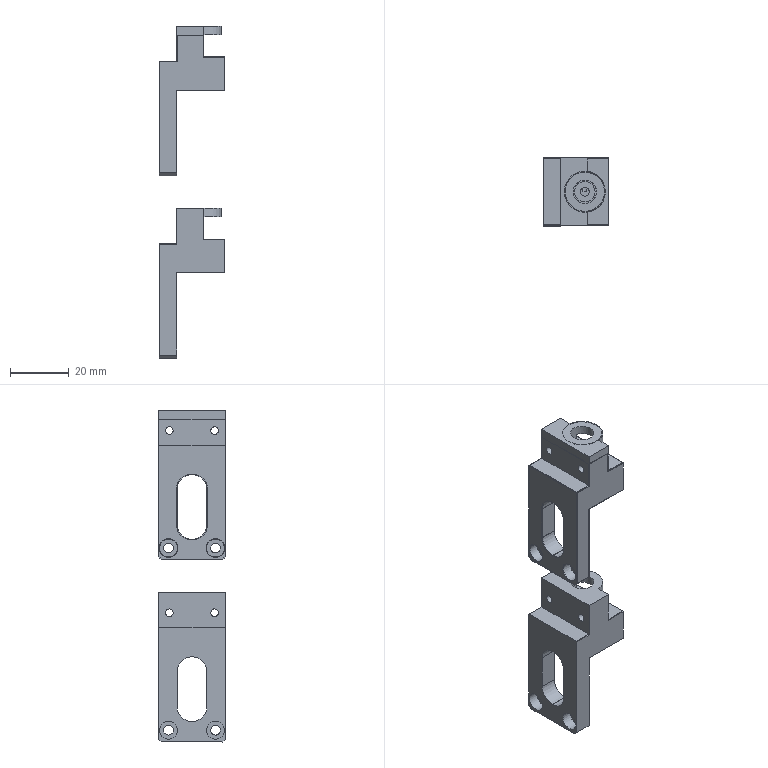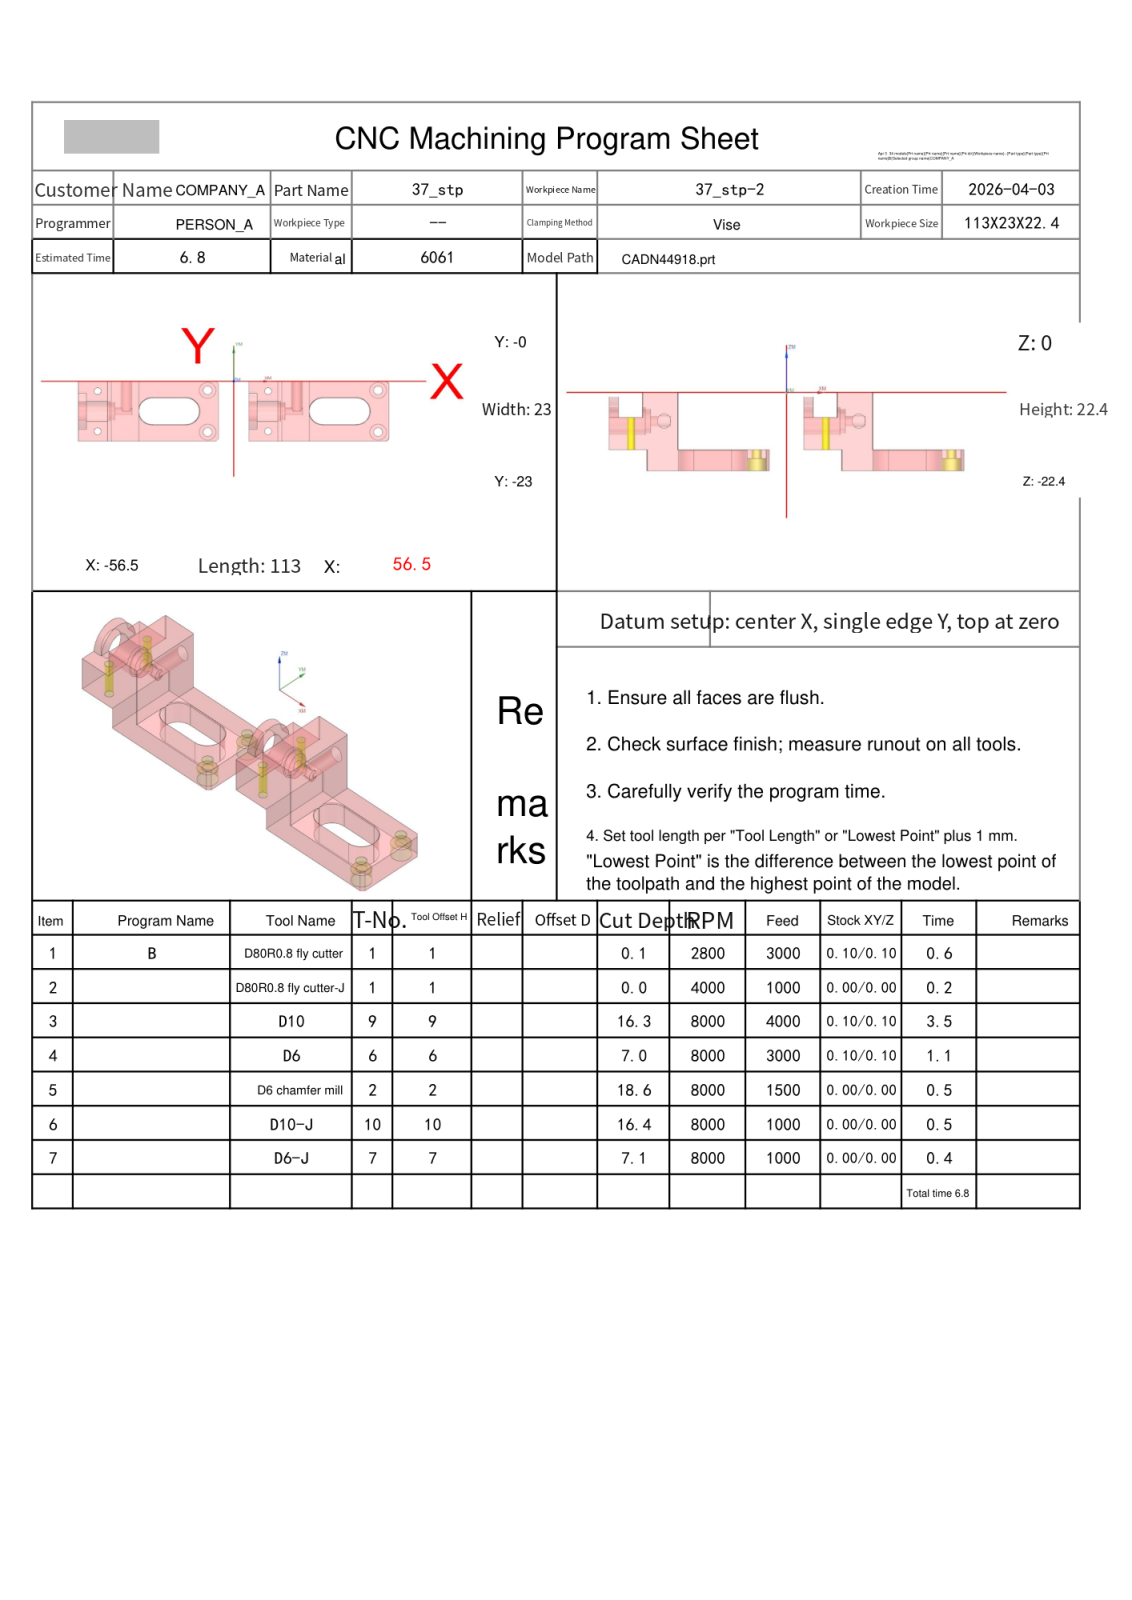NC program | NX | posted by the shop | part box 22.4 x 23 x 113 mm
Lines 1 to 3243 of 3535, first 2166 of 3241 lines:
%
O0001
(Machine time: 8.11 MIN)
(===Total Tool:6===)
(T1=D80R0.8 fly cutter D=80.  R=0.8  D-  H01 Z=-0.   )
(T9=D10     D=10.  R=0.   D-  H09 Z=-16.3 )
(T6=D6      D=6.   R=0.   D-  H06 Z=-7.05 )
(T2=D6 chamfer mill   D=6.   R=0.   D-  H02 Z=-18.6 )
(T10=D10-J  D=10.  R=0.   D10 H10 Z=-16.4 )
(T7=D6-J    D=6.   R=0.   D7  H07 Z=-7.15 )
G80 G90 G17 G49 G40
G91 G28 Z0
M01
N1 T01 M06
(D80R0.8 fly cutter  D=80. R=0.8 H=01 ce=0.10 di=0.10)
G00 G90 G54 X-108.597 Y-11.5 M03 S2800
G43 H01 Z20.
M08
Z4.517
G01 Z2.517 F3000.
X-96.597
X96.597
X108.597
Z4.517
G00 X-108.597
Z4.033
G01 Z2.033
X-96.597
X96.597
X108.597
Z4.033
G00 X-108.597
Z3.55
G01 Z1.55
X-96.597
X96.597
X108.597
Z3.55
G00 X-108.597
Z3.067
G01 Z1.067
X-96.597
X96.597
X108.597
Z3.067
G00 Z20.
X-108.597
Z2.583
G01 Z.583
X-96.597
X96.597
X108.597
Z2.583
G00 Z20.
X-108.597
Z2.1
G01 Z.1
X-96.597
X96.597
X108.597
Z2.1
G00 Z20.
G91 G28 Z0.0
M05
M09
G91 G28 Z0.0
M01
N2 T01 M06
(D80R0.8 fly cutter-J  D=80. R=0.8 H=01 ce=0.00 di=0.00)
G00 G90 G54 X-108.499 Y-11.5 M03 S4000
G43 H01 Z20.
M08
Z2.
G01 Z0.0 F1000.
X-96.499
X96.499
X108.499
Z2.
G00 Z20.
G91 G28 Z0.0
M05
M09
G91 G28 Z0.0
M01
N3 T09 M06
(D10  D=10. R=0. H=09 ce=0.10 di=0.10)
G00 G90 G54 X64.5 Y-11.5 M03 S8000
G43 H09 Z12.4
M08
Z.918
G01 Z-.582 F4000.
X61.4
Y-24.03
X57.53 Y-27.9
X29.612
X32.6 Y-24.912
Y-11.9
X44.5
G03 X44.8 Y-11.6 I0.0 J.3
G01 Y-11.4
G03 X44.5 Y-11.1 I-.3 J0.0
G01 X32.6
Y1.912
X29.612 Y4.9
X57.53
X61.4 Y1.03
Y-8.465
G02 X60.955 Y-9.297 I-1. J0.0
G01 X54.345 Y-13.703
G03 X53.9 Y-14.535 I.555 J-.832
G01 Y-19.401
G02 X52.901 Y-20.4 I-1. J.001
G01 X40.599
G02 X40.1 Y-19.9 I.001 J.5
X40.599 Y-19.4 I.5 J0.0
G01 X44.5
G03 X52.3 Y-11.6 I0.0 J7.8
X52.303 Y-11.4 I-7.797 J.2
X44.503 Y-3.6 I-7.8 J0.0
G01 X44.5
X40.599
G02 X40.1 Y-3.1 I.001 J.5
X40.599 Y-2.6 I.5 J0.0
G01 X52.901
G02 X53.9 Y-3.599 I-.001 J-1.
G01 Y-11.5
Y-12.
X64.5
Z.918
G00 Y-11.5
Z.336
G01 Z-1.164
X61.4
Y-24.03
X57.53 Y-27.9
X29.612
X32.6 Y-24.912
Y-11.9
X44.5
G03 X44.8 Y-11.6 I0.0 J.3
G01 Y-11.4
G03 X44.5 Y-11.1 I-.3 J0.0
G01 X32.6
Y1.912
X29.612 Y4.9
X57.53
X61.4 Y1.03
Y-8.465
G02 X60.955 Y-9.297 I-1. J0.0
G01 X54.345 Y-13.703
G03 X53.9 Y-14.535 I.555 J-.832
G01 Y-19.401
G02 X52.901 Y-20.4 I-1. J.001
G01 X40.599
G02 X40.1 Y-19.9 I.001 J.5
X40.599 Y-19.4 I.5 J0.0
G01 X44.5
G03 X52.3 Y-11.6 I0.0 J7.8
X52.303 Y-11.4 I-7.797 J.2
X44.503 Y-3.6 I-7.8 J0.0
G01 X44.5
X40.599
G02 X40.1 Y-3.1 I.001 J.5
X40.599 Y-2.6 I.5 J0.0
G01 X52.901
G02 X53.9 Y-3.599 I-.001 J-1.
G01 Y-11.5
Y-12.
X64.5
Z.336
G00 Y-11.5
Z-.246
G01 Z-1.746
X61.4
Y-24.03
X57.53 Y-27.9
X29.612
X32.6 Y-24.912
Y-11.9
X44.5
G03 X44.8 Y-11.6 I0.0 J.3
G01 Y-11.4
G03 X44.5 Y-11.1 I-.3 J0.0
G01 X32.6
Y1.912
X29.612 Y4.9
X57.53
X61.4 Y1.03
Y-8.465
G02 X60.955 Y-9.297 I-1. J0.0
G01 X54.345 Y-13.703
G03 X53.9 Y-14.535 I.555 J-.832
G01 Y-19.401
G02 X52.901 Y-20.4 I-1. J.001
G01 X40.599
G02 X40.1 Y-19.9 I.001 J.5
X40.599 Y-19.4 I.5 J0.0
G01 X44.5
G03 X52.3 Y-11.6 I0.0 J7.8
X52.303 Y-11.4 I-7.797 J.2
X44.503 Y-3.6 I-7.8 J0.0
G01 X44.5
X40.599
G02 X40.1 Y-3.1 I.001 J.5
X40.599 Y-2.6 I.5 J0.0
G01 X52.901
G02 X53.9 Y-3.599 I-.001 J-1.
G01 Y-11.5
Y-12.
X64.5
Z-.246
G00 Y-11.5
Z-.829
G01 Z-2.329
X61.4
Y-24.03
X57.53 Y-27.9
X29.612
X32.6 Y-24.912
Y-11.9
X44.5
G03 X44.8 Y-11.6 I0.0 J.3
G01 Y-11.4
G03 X44.5 Y-11.1 I-.3 J0.0
G01 X32.6
Y1.912
X29.612 Y4.9
X57.53
X61.4 Y1.03
Y-8.465
G02 X60.955 Y-9.297 I-1. J0.0
G01 X54.345 Y-13.703
G03 X53.9 Y-14.535 I.555 J-.832
G01 Y-19.401
G02 X52.901 Y-20.4 I-1. J.001
G01 X40.599
G02 X40.1 Y-19.9 I.001 J.5
X40.599 Y-19.4 I.5 J0.0
G01 X44.5
G03 X52.3 Y-11.6 I0.0 J7.8
X52.303 Y-11.4 I-7.797 J.2
X44.503 Y-3.6 I-7.8 J0.0
G01 X44.5
X40.599
G02 X40.1 Y-3.1 I.001 J.5
X40.599 Y-2.6 I.5 J0.0
G01 X52.901
G02 X53.9 Y-3.599 I-.001 J-1.
G01 Y-11.5
Y-12.
X64.5
Z-.829
G00 Y-11.5
Z-1.411
G01 Z-2.911
X61.4
Y-24.03
X57.53 Y-27.9
X29.612
X32.6 Y-24.912
Y-11.9
X44.5
G03 X44.8 Y-11.6 I0.0 J.3
G01 Y-11.4
G03 X44.5 Y-11.1 I-.3 J0.0
G01 X32.6
Y1.912
X29.612 Y4.9
X57.53
X61.4 Y1.03
Y-8.465
G02 X60.955 Y-9.297 I-1. J0.0
G01 X54.345 Y-13.703
G03 X53.9 Y-14.535 I.555 J-.832
G01 Y-19.401
G02 X52.901 Y-20.4 I-1. J.001
G01 X40.599
G02 X40.1 Y-19.9 I.001 J.5
X40.599 Y-19.4 I.5 J0.0
G01 X44.5
G03 X52.3 Y-11.6 I0.0 J7.8
X52.303 Y-11.4 I-7.797 J.2
X44.503 Y-3.6 I-7.8 J0.0
G01 X44.5
X40.599
G02 X40.1 Y-3.1 I.001 J.5
X40.599 Y-2.6 I.5 J0.0
G01 X52.901
G02 X53.9 Y-3.599 I-.001 J-1.
G01 Y-11.5
Y-12.
X64.5
Z-1.411
G00 Y-11.5
Z-1.993
G01 Z-3.493
X61.4
Y-24.03
X57.53 Y-27.9
X29.612
X32.6 Y-24.912
Y-11.9
X44.5
G03 X44.8 Y-11.6 I0.0 J.3
G01 Y-11.4
G03 X44.5 Y-11.1 I-.3 J0.0
G01 X32.6
Y1.912
X29.612 Y4.9
X57.53
X61.4 Y1.03
Y-8.465
G02 X60.955 Y-9.297 I-1. J0.0
G01 X54.345 Y-13.703
G03 X53.9 Y-14.535 I.555 J-.832
G01 Y-19.401
G02 X52.901 Y-20.4 I-1. J.001
G01 X40.599
G02 X40.1 Y-19.9 I.001 J.5
X40.599 Y-19.4 I.5 J0.0
G01 X44.5
G03 X52.3 Y-11.6 I0.0 J7.8
X52.303 Y-11.4 I-7.797 J.2
X44.503 Y-3.6 I-7.8 J0.0
G01 X44.5
X40.599
G02 X40.1 Y-3.1 I.001 J.5
X40.599 Y-2.6 I.5 J0.0
G01 X52.901
G02 X53.9 Y-3.599 I-.001 J-1.
G01 Y-11.5
Y-12.
X64.5
Z-1.993
G00 Y-11.5
Z-2.575
G01 Z-4.075
X61.4
Y-24.03
X57.53 Y-27.9
X29.612
X32.6 Y-24.912
Y-11.9
X44.5
G03 X44.8 Y-11.6 I0.0 J.3
G01 Y-11.4
G03 X44.5 Y-11.1 I-.3 J0.0
G01 X32.6
Y1.912
X29.612 Y4.9
X57.53
X61.4 Y1.03
Y-8.465
G02 X60.955 Y-9.297 I-1. J0.0
G01 X54.345 Y-13.703
G03 X53.9 Y-14.535 I.555 J-.832
G01 Y-19.401
G02 X52.901 Y-20.4 I-1. J.001
G01 X40.599
G02 X40.1 Y-19.9 I.001 J.5
X40.599 Y-19.4 I.5 J0.0
G01 X44.5
G03 X52.3 Y-11.6 I0.0 J7.8
X52.303 Y-11.4 I-7.797 J.2
X44.503 Y-3.6 I-7.8 J0.0
G01 X44.5
X40.599
G02 X40.1 Y-3.1 I.001 J.5
X40.599 Y-2.6 I.5 J0.0
G01 X52.901
G02 X53.9 Y-3.599 I-.001 J-1.
G01 Y-11.5
Y-12.
X64.5
Z-2.575
G00 Y-11.5
Z-3.157
G01 Z-4.657
X61.4
Y-24.03
X57.53 Y-27.9
X29.612
X32.6 Y-24.912
Y-11.9
X44.5
G03 X44.8 Y-11.6 I0.0 J.3
G01 Y-11.4
G03 X44.5 Y-11.1 I-.3 J0.0
G01 X32.6
Y1.912
X29.612 Y4.9
X57.53
X61.4 Y1.03
Y-8.465
G02 X60.955 Y-9.297 I-1. J0.0
G01 X54.345 Y-13.703
G03 X53.9 Y-14.535 I.555 J-.832
G01 Y-19.401
G02 X52.901 Y-20.4 I-1. J.001
G01 X40.599
G02 X40.1 Y-19.9 I.001 J.5
X40.599 Y-19.4 I.5 J0.0
G01 X44.5
G03 X52.3 Y-11.6 I0.0 J7.8
X52.303 Y-11.4 I-7.797 J.2
X44.503 Y-3.6 I-7.8 J0.0
G01 X44.5
X40.599
G02 X40.1 Y-3.1 I.001 J.5
X40.599 Y-2.6 I.5 J0.0
G01 X52.901
G02 X53.9 Y-3.599 I-.001 J-1.
G01 Y-11.5
Y-12.
X64.5
Z-3.157
G00 Y-11.5
Z-3.739
G01 Z-5.239
X61.4
Y-24.03
X57.53 Y-27.9
X29.612
X32.6 Y-24.912
Y-11.9
X44.5
G03 X44.8 Y-11.6 I0.0 J.3
G01 Y-11.4
G03 X44.5 Y-11.1 I-.3 J0.0
G01 X32.6
Y1.912
X29.612 Y4.9
X57.53
X61.4 Y1.03
Y-8.465
G02 X60.955 Y-9.297 I-1. J0.0
G01 X54.345 Y-13.703
G03 X53.9 Y-14.535 I.555 J-.832
G01 Y-19.401
G02 X52.901 Y-20.4 I-1. J.001
G01 X40.599
G02 X40.1 Y-19.9 I.001 J.5
X40.599 Y-19.4 I.5 J0.0
G01 X44.5
G03 X52.3 Y-11.6 I0.0 J7.8
X52.303 Y-11.4 I-7.797 J.2
X44.503 Y-3.6 I-7.8 J0.0
G01 X44.5
X40.599
G02 X40.1 Y-3.1 I.001 J.5
X40.599 Y-2.6 I.5 J0.0
G01 X52.901
G02 X53.9 Y-3.599 I-.001 J-1.
G01 Y-11.5
Y-12.
X64.5
Z-3.739
G00 Y-11.5
Z-4.321
G01 Z-5.821
X61.4
Y-24.03
X57.53 Y-27.9
X29.612
X32.6 Y-24.912
Y-11.9
X44.5
G03 X44.8 Y-11.6 I0.0 J.3
G01 Y-11.4
G03 X44.5 Y-11.1 I-.3 J0.0
G01 X32.6
Y1.912
X29.612 Y4.9
X57.53
X61.4 Y1.03
Y-8.465
G02 X60.955 Y-9.297 I-1. J0.0
G01 X54.345 Y-13.703
G03 X53.9 Y-14.535 I.555 J-.832
G01 Y-19.401
G02 X52.901 Y-20.4 I-1. J.001
G01 X40.599
G02 X40.1 Y-19.9 I.001 J.5
X40.599 Y-19.4 I.5 J0.0
G01 X44.5
G03 X52.3 Y-11.6 I0.0 J7.8
X52.303 Y-11.4 I-7.797 J.2
X44.503 Y-3.6 I-7.8 J0.0
G01 X44.5
X40.599
G02 X40.1 Y-3.1 I.001 J.5
X40.599 Y-2.6 I.5 J0.0
G01 X52.901
G02 X53.9 Y-3.599 I-.001 J-1.
G01 Y-11.5
Y-12.
X64.5
Z-4.321
G00 Y-11.5
Z-4.904
G01 Z-6.404
X61.4
Y-24.03
X57.53 Y-27.9
X29.612
X32.6 Y-24.912
Y-11.9
X44.5
G03 X44.8 Y-11.6 I0.0 J.3
G01 Y-11.4
G03 X44.5 Y-11.1 I-.3 J0.0
G01 X32.6
Y1.912
X29.612 Y4.9
X57.53
X61.4 Y1.03
Y-8.465
G02 X60.955 Y-9.297 I-1. J0.0
G01 X54.345 Y-13.703
G03 X53.9 Y-14.535 I.555 J-.832
G01 Y-19.401
G02 X52.901 Y-20.4 I-1. J.001
G01 X40.599
G02 X40.1 Y-19.9 I.001 J.5
X40.599 Y-19.4 I.5 J0.0
G01 X44.5
G03 X52.3 Y-11.6 I0.0 J7.8
X52.303 Y-11.4 I-7.797 J.2
X44.503 Y-3.6 I-7.8 J0.0
G01 X44.5
X40.599
G02 X40.1 Y-3.1 I.001 J.5
X40.599 Y-2.6 I.5 J0.0
G01 X52.901
G02 X53.9 Y-3.599 I-.001 J-1.
G01 Y-11.5
Y-12.
X64.5
Z-4.904
G00 Y-11.5
Z-5.486
G01 Z-6.986
X61.4
Y-24.03
X57.53 Y-27.9
X29.612
X32.6 Y-24.912
Y-11.9
X44.5
G03 X44.8 Y-11.6 I0.0 J.3
G01 Y-11.4
G03 X44.5 Y-11.1 I-.3 J0.0
G01 X32.6
Y1.912
X29.612 Y4.9
X57.53
X61.4 Y1.03
Y-8.465
G02 X60.955 Y-9.297 I-1. J0.0
G01 X54.345 Y-13.703
G03 X53.9 Y-14.535 I.555 J-.832
G01 Y-19.401
G02 X52.901 Y-20.4 I-1. J.001
G01 X40.599
G02 X40.1 Y-19.9 I.001 J.5
X40.599 Y-19.4 I.5 J0.0
G01 X44.5
G03 X52.3 Y-11.6 I0.0 J7.8
X52.303 Y-11.4 I-7.797 J.2
X44.503 Y-3.6 I-7.8 J0.0
G01 X44.5
X40.599
G02 X40.1 Y-3.1 I.001 J.5
X40.599 Y-2.6 I.5 J0.0
G01 X52.901
G02 X53.9 Y-3.599 I-.001 J-1.
G01 Y-11.5
Y-12.
X64.5
Z-5.486
G00 Y-11.5
Z-6.068
G01 Z-7.568
X61.4
Y-24.03
X57.53 Y-27.9
X29.612
X32.6 Y-24.912
Y-11.9
X44.5
G03 X44.8 Y-11.6 I0.0 J.3
G01 Y-11.4
G03 X44.5 Y-11.1 I-.3 J0.0
G01 X32.6
Y1.912
X29.612 Y4.9
X57.53
X61.4 Y1.03
Y-8.465
G02 X60.955 Y-9.297 I-1. J0.0
G01 X54.345 Y-13.703
G03 X53.9 Y-14.535 I.555 J-.832
G01 Y-19.401
G02 X52.901 Y-20.4 I-1. J.001
G01 X40.599
G02 X40.1 Y-19.9 I.001 J.5
X40.599 Y-19.4 I.5 J0.0
G01 X44.5
G03 X52.3 Y-11.6 I0.0 J7.8
X52.303 Y-11.4 I-7.797 J.2
X44.503 Y-3.6 I-7.8 J0.0
G01 X44.5
X40.599
G02 X40.1 Y-3.1 I.001 J.5
X40.599 Y-2.6 I.5 J0.0
G01 X52.901
G02 X53.9 Y-3.599 I-.001 J-1.
G01 Y-11.5
Y-12.
X64.5
Z-6.068
G00 Y-11.5
Z-6.65
G01 Z-8.15
X61.4
Y-24.03
X57.53 Y-27.9
X29.612
X32.6 Y-24.912
Y-11.9
X44.5
G03 X44.8 Y-11.6 I0.0 J.3
G01 Y-11.4
G03 X44.5 Y-11.1 I-.3 J0.0
G01 X32.6
Y1.912
X29.612 Y4.9
X57.53
X61.4 Y1.03
Y-8.465
G02 X60.955 Y-9.297 I-1. J0.0
G01 X54.345 Y-13.703
G03 X53.9 Y-14.535 I.555 J-.832
G01 Y-19.401
G02 X52.901 Y-20.4 I-1. J.001
G01 X40.599
G02 X40.1 Y-19.9 I.001 J.5
X40.599 Y-19.4 I.5 J0.0
G01 X44.5
G03 X52.3 Y-11.6 I0.0 J7.8
X52.303 Y-11.4 I-7.797 J.2
X44.503 Y-3.6 I-7.8 J0.0
G01 X44.5
X40.599
G02 X40.1 Y-3.1 I.001 J.5
X40.599 Y-2.6 I.5 J0.0
G01 X52.901
G02 X53.9 Y-3.599 I-.001 J-1.
G01 Y-11.5
Y-12.
X64.5
Z-6.65
G00 Y-11.5
Z-7.232
G01 Z-8.732
X61.4
Y-24.03
X57.53 Y-27.9
X29.612
X32.6 Y-24.912
Y-11.9
X44.5
G03 X44.8 Y-11.6 I0.0 J.3
G01 Y-11.4
G03 X44.5 Y-11.1 I-.3 J0.0
G01 X32.6
Y1.912
X29.612 Y4.9
X57.53
X61.4 Y1.03
Y-8.465
G02 X60.955 Y-9.297 I-1. J0.0
G01 X54.345 Y-13.703
G03 X53.9 Y-14.535 I.555 J-.832
G01 Y-19.401
G02 X52.901 Y-20.4 I-1. J.001
G01 X40.599
G02 X40.1 Y-19.9 I.001 J.5
X40.599 Y-19.4 I.5 J0.0
G01 X44.5
G03 X52.3 Y-11.6 I0.0 J7.8
X52.303 Y-11.4 I-7.797 J.2
X44.503 Y-3.6 I-7.8 J0.0
G01 X44.5
X40.599
G02 X40.1 Y-3.1 I.001 J.5
X40.599 Y-2.6 I.5 J0.0
G01 X52.901
G02 X53.9 Y-3.599 I-.001 J-1.
G01 Y-11.5
Y-12.
X64.5
Z-7.232
G00 Y-11.5
Z-7.814
G01 Z-9.314
X61.4
Y-24.03
X57.53 Y-27.9
X29.612
X32.6 Y-24.912
Y-11.9
X44.5
G03 X44.8 Y-11.6 I0.0 J.3
G01 Y-11.4
G03 X44.5 Y-11.1 I-.3 J0.0
G01 X32.6
Y1.912
X29.612 Y4.9
X57.53
X61.4 Y1.03
Y-8.465
G02 X60.955 Y-9.297 I-1. J0.0
G01 X54.345 Y-13.703
G03 X53.9 Y-14.535 I.555 J-.832
G01 Y-19.401
G02 X52.901 Y-20.4 I-1. J.001
G01 X40.599
G02 X40.1 Y-19.9 I.001 J.5
X40.599 Y-19.4 I.5 J0.0
G01 X44.5
G03 X52.3 Y-11.6 I0.0 J7.8
X52.303 Y-11.4 I-7.797 J.2
X44.503 Y-3.6 I-7.8 J0.0
G01 X44.5
X40.599
G02 X40.1 Y-3.1 I.001 J.5
X40.599 Y-2.6 I.5 J0.0
G01 X52.901
G02 X53.9 Y-3.599 I-.001 J-1.
G01 Y-11.5
Y-12.
X64.5
Z-7.814
G00 Y-11.5
Z-8.396
G01 Z-9.896
X61.4
Y-24.03
X57.53 Y-27.9
X29.612
X32.6 Y-24.912
Y-11.9
X44.5
G03 X44.8 Y-11.6 I0.0 J.3
G01 Y-11.4
G03 X44.5 Y-11.1 I-.3 J0.0
G01 X32.6
Y1.912
X29.612 Y4.9
X57.53
X61.4 Y1.03
Y-8.465
G02 X60.955 Y-9.297 I-1. J0.0
G01 X54.345 Y-13.703
G03 X53.9 Y-14.535 I.555 J-.832
G01 Y-19.401
G02 X52.901 Y-20.4 I-1. J.001
G01 X40.599
G02 X40.1 Y-19.9 I.001 J.5
X40.599 Y-19.4 I.5 J0.0
G01 X44.5
G03 X52.3 Y-11.6 I0.0 J7.8
X52.303 Y-11.4 I-7.797 J.2
X44.503 Y-3.6 I-7.8 J0.0
G01 X44.5
X40.599
G02 X40.1 Y-3.1 I.001 J.5
X40.599 Y-2.6 I.5 J0.0
G01 X52.901
G02 X53.9 Y-3.599 I-.001 J-1.
G01 Y-11.5
Y-12.
X64.5
Z-8.396
G00 Y-11.5
Z-8.979
G01 Z-10.479
X61.4
Y-24.03
X57.53 Y-27.9
X29.612
X32.6 Y-24.912
Y-11.9
X44.5
G03 X44.8 Y-11.6 I0.0 J.3
G01 Y-11.4
G03 X44.5 Y-11.1 I-.3 J0.0
G01 X32.6
Y1.912
X29.612 Y4.9
X57.53
X61.4 Y1.03
Y-8.465
G02 X60.955 Y-9.297 I-1. J0.0
G01 X54.345 Y-13.703
G03 X53.9 Y-14.535 I.555 J-.832
G01 Y-19.401
G02 X52.901 Y-20.4 I-1. J.001
G01 X40.599
G02 X40.1 Y-19.9 I.001 J.5
X40.599 Y-19.4 I.5 J0.0
G01 X44.5
G03 X52.3 Y-11.6 I0.0 J7.8
X52.303 Y-11.4 I-7.797 J.2
X44.503 Y-3.6 I-7.8 J0.0
G01 X44.5
X40.599
G02 X40.1 Y-3.1 I.001 J.5
X40.599 Y-2.6 I.5 J0.0
G01 X52.901
G02 X53.9 Y-3.599 I-.001 J-1.
G01 Y-11.5
Y-12.
X64.5
Z-8.979
G00 Y-11.5
Z-9.561
G01 Z-11.061
X61.4
Y-24.03
X57.53 Y-27.9
X29.612
X32.6 Y-24.912
Y-11.9
X44.5
G03 X44.8 Y-11.6 I0.0 J.3
G01 Y-11.4
G03 X44.5 Y-11.1 I-.3 J0.0
G01 X32.6
Y1.912
X29.612 Y4.9
X57.53
X61.4 Y1.03
Y-8.465
G02 X60.955 Y-9.297 I-1. J0.0
G01 X54.345 Y-13.703
G03 X53.9 Y-14.535 I.555 J-.832
G01 Y-19.401
G02 X52.901 Y-20.4 I-1. J.001
G01 X40.599
G02 X40.1 Y-19.9 I.001 J.5
X40.599 Y-19.4 I.5 J0.0
G01 X44.5
G03 X52.3 Y-11.6 I0.0 J7.8
X52.303 Y-11.4 I-7.797 J.2
X44.503 Y-3.6 I-7.8 J0.0
G01 X44.5
X40.599
G02 X40.1 Y-3.1 I.001 J.5
X40.599 Y-2.6 I.5 J0.0
G01 X52.901
G02 X53.9 Y-3.599 I-.001 J-1.
G01 Y-11.5
Y-12.
X64.5
Z-9.561
G00 Y-11.5
Z-10.143
G01 Z-11.643
X61.4
Y-24.03
X57.53 Y-27.9
X29.612
X32.6 Y-24.912
Y-11.9
X44.5
G03 X44.8 Y-11.6 I0.0 J.3
G01 Y-11.4
G03 X44.5 Y-11.1 I-.3 J0.0
G01 X32.6
Y1.912
X29.612 Y4.9
X57.53
X61.4 Y1.03
Y-8.465
G02 X60.955 Y-9.297 I-1. J0.0
G01 X54.345 Y-13.703
G03 X53.9 Y-14.535 I.555 J-.832
G01 Y-19.401
G02 X52.901 Y-20.4 I-1. J.001
G01 X40.599
G02 X40.1 Y-19.9 I.001 J.5
X40.599 Y-19.4 I.5 J0.0
G01 X44.5
G03 X52.3 Y-11.6 I0.0 J7.8
X52.303 Y-11.4 I-7.797 J.2
X44.503 Y-3.6 I-7.8 J0.0
G01 X44.5
X40.599
G02 X40.1 Y-3.1 I.001 J.5
X40.599 Y-2.6 I.5 J0.0
G01 X52.901
G02 X53.9 Y-3.599 I-.001 J-1.
G01 Y-11.5
Y-12.
X64.5
Z-10.143
G00 Y-11.5
Z-10.725
G01 Z-12.225
X61.4
Y-24.03
X57.53 Y-27.9
X29.612
X32.6 Y-24.912
Y-11.9
X44.5
G03 X44.8 Y-11.6 I0.0 J.3
G01 Y-11.4
G03 X44.5 Y-11.1 I-.3 J0.0
G01 X32.6
Y1.912
X29.612 Y4.9
X57.53
X61.4 Y1.03
Y-8.465
G02 X60.955 Y-9.297 I-1. J0.0
G01 X54.345 Y-13.703
G03 X53.9 Y-14.535 I.555 J-.832
G01 Y-19.401
G02 X52.901 Y-20.4 I-1. J.001
G01 X40.599
G02 X40.1 Y-19.9 I.001 J.5
X40.599 Y-19.4 I.5 J0.0
G01 X44.5
G03 X52.3 Y-11.6 I0.0 J7.8
X52.303 Y-11.4 I-7.797 J.2
X44.503 Y-3.6 I-7.8 J0.0
G01 X44.5
X40.599
G02 X40.1 Y-3.1 I.001 J.5
X40.599 Y-2.6 I.5 J0.0
G01 X52.901
G02 X53.9 Y-3.599 I-.001 J-1.
G01 Y-11.5
Y-12.
X64.5
Z-10.725
G00 Y-11.5
Z-11.307
G01 Z-12.807
X61.4
Y-24.03
X57.53 Y-27.9
X29.612
X32.6 Y-24.912
Y-11.9
X44.5
G03 X44.8 Y-11.6 I0.0 J.3
G01 Y-11.4
G03 X44.5 Y-11.1 I-.3 J0.0
G01 X32.6
Y1.912
X29.612 Y4.9
X57.53
X61.4 Y1.03
Y-8.465
G02 X60.955 Y-9.297 I-1. J0.0
G01 X54.345 Y-13.703
G03 X53.9 Y-14.535 I.555 J-.832
G01 Y-19.401
G02 X52.901 Y-20.4 I-1. J.001
G01 X40.599
G02 X40.1 Y-19.9 I.001 J.5
X40.599 Y-19.4 I.5 J0.0
G01 X44.5
G03 X52.3 Y-11.6 I0.0 J7.8
X52.303 Y-11.4 I-7.797 J.2
X44.503 Y-3.6 I-7.8 J0.0
G01 X44.5
X40.599
G02 X40.1 Y-3.1 I.001 J.5
X40.599 Y-2.6 I.5 J0.0
G01 X52.901
G02 X53.9 Y-3.599 I-.001 J-1.
G01 Y-11.5
Y-12.
X64.5
Z-11.307
G00 Y-11.5
Z-11.889
G01 Z-13.389
X61.4
Y-24.03
X57.53 Y-27.9
X29.612
X32.6 Y-24.912
Y-11.9
X44.5
G03 X44.8 Y-11.6 I0.0 J.3
G01 Y-11.4
G03 X44.5 Y-11.1 I-.3 J0.0
G01 X32.6
Y1.912
X29.612 Y4.9
X57.53
X61.4 Y1.03
Y-8.465
G02 X60.955 Y-9.297 I-1. J0.0
G01 X54.345 Y-13.703
G03 X53.9 Y-14.535 I.555 J-.832
G01 Y-19.401
G02 X52.901 Y-20.4 I-1. J.001
G01 X40.599
G02 X40.1 Y-19.9 I.001 J.5
X40.599 Y-19.4 I.5 J0.0
G01 X44.5
G03 X52.3 Y-11.6 I0.0 J7.8
X52.303 Y-11.4 I-7.797 J.2
X44.503 Y-3.6 I-7.8 J0.0
G01 X44.5
X40.599
G02 X40.1 Y-3.1 I.001 J.5
X40.599 Y-2.6 I.5 J0.0
G01 X52.901
G02 X53.9 Y-3.599 I-.001 J-1.
G01 Y-11.5
Y-12.
X64.5
Z-11.889
G00 Y-11.5
Z-12.471
G01 Z-13.971
X61.4
Y-24.03
X57.53 Y-27.9
X29.612
X32.6 Y-24.912
Y-11.9
X44.5
G03 X44.8 Y-11.6 I0.0 J.3
G01 Y-11.4
G03 X44.5 Y-11.1 I-.3 J0.0
G01 X32.6
Y1.912
X29.612 Y4.9
X57.53
X61.4 Y1.03
Y-8.465
G02 X60.955 Y-9.297 I-1. J0.0
G01 X54.345 Y-13.703
G03 X53.9 Y-14.535 I.555 J-.832
G01 Y-19.401
G02 X52.901 Y-20.4 I-1. J.001
G01 X40.599
G02 X40.1 Y-19.9 I.001 J.5
X40.599 Y-19.4 I.5 J0.0
G01 X44.5
G03 X52.3 Y-11.6 I0.0 J7.8
X52.303 Y-11.4 I-7.797 J.2
X44.503 Y-3.6 I-7.8 J0.0
G01 X44.5
X40.599
G02 X40.1 Y-3.1 I.001 J.5
X40.599 Y-2.6 I.5 J0.0
G01 X52.901
G02 X53.9 Y-3.599 I-.001 J-1.
G01 Y-11.5
Y-12.
X64.5
Z-12.471
G00 Y-11.5
Z-13.054
G01 Z-14.554
X61.4
Y-24.03
X57.53 Y-27.9
X29.612
X32.6 Y-24.912
Y-11.9
X44.5
G03 X44.8 Y-11.6 I0.0 J.3
G01 Y-11.4
G03 X44.5 Y-11.1 I-.3 J0.0
G01 X32.6
Y1.912
X29.612 Y4.9
X57.53
X61.4 Y1.03
Y-8.465
G02 X60.955 Y-9.297 I-1. J0.0
G01 X54.345 Y-13.703
G03 X53.9 Y-14.535 I.555 J-.832
G01 Y-19.401
G02 X52.901 Y-20.4 I-1. J.001
G01 X40.599
G02 X40.1 Y-19.9 I.001 J.5
X40.599 Y-19.4 I.5 J0.0
G01 X44.5
G03 X52.3 Y-11.6 I0.0 J7.8
X52.303 Y-11.4 I-7.797 J.2
X44.503 Y-3.6 I-7.8 J0.0
G01 X44.5
X40.599
G02 X40.1 Y-3.1 I.001 J.5
X40.599 Y-2.6 I.5 J0.0
G01 X52.901
G02 X53.9 Y-3.599 I-.001 J-1.
G01 Y-11.5
Y-12.
X64.5
Z-13.054
G00 Y-11.5
Z-13.636
G01 Z-15.136
X61.4
Y-24.03
X57.53 Y-27.9
X29.612
X32.6 Y-24.912
Y-11.9
X44.5
G03 X44.8 Y-11.6 I0.0 J.3
G01 Y-11.4
G03 X44.5 Y-11.1 I-.3 J0.0
G01 X32.6
Y1.912
X29.612 Y4.9
X57.53
X61.4 Y1.03
Y-8.465
G02 X60.955 Y-9.297 I-1. J0.0
G01 X54.345 Y-13.703
G03 X53.9 Y-14.535 I.555 J-.832
G01 Y-19.401
G02 X52.901 Y-20.4 I-1. J.001
G01 X40.599
G02 X40.1 Y-19.9 I.001 J.5
X40.599 Y-19.4 I.5 J0.0
G01 X44.5
G03 X52.3 Y-11.6 I0.0 J7.8
X52.303 Y-11.4 I-7.797 J.2
X44.503 Y-3.6 I-7.8 J0.0
G01 X44.5
X40.599
G02 X40.1 Y-3.1 I.001 J.5
X40.599 Y-2.6 I.5 J0.0
G01 X52.901
G02 X53.9 Y-3.599 I-.001 J-1.
G01 Y-11.5
Y-12.
X64.5
Z-13.636
G00 Y-11.5
Z-14.218
G01 Z-15.718
X61.4
Y-24.03
X57.53 Y-27.9
X29.612
X32.6 Y-24.912
Y-11.9
X44.5
G03 X44.8 Y-11.6 I0.0 J.3
G01 Y-11.4
G03 X44.5 Y-11.1 I-.3 J0.0
G01 X32.6
Y1.912
X29.612 Y4.9
X57.53
X61.4 Y1.03
Y-8.465
G02 X60.955 Y-9.297 I-1. J0.0
G01 X54.345 Y-13.703
G03 X53.9 Y-14.535 I.555 J-.832
G01 Y-19.401
G02 X52.901 Y-20.4 I-1. J.001
G01 X40.599
G02 X40.1 Y-19.9 I.001 J.5
X40.599 Y-19.4 I.5 J0.0
G01 X44.5
G03 X52.3 Y-11.6 I0.0 J7.8
X52.303 Y-11.4 I-7.797 J.2
X44.503 Y-3.6 I-7.8 J0.0
G01 X44.5
X40.599
G02 X40.1 Y-3.1 I.001 J.5
X40.599 Y-2.6 I.5 J0.0
G01 X52.901
G02 X53.9 Y-3.599 I-.001 J-1.
G01 Y-11.5
Y-12.
X64.5
Z-14.218
G00 Y-11.5
Z-14.8
G01 Z-16.3
X61.4
Y-24.03
X57.53 Y-27.9
X29.612
X32.6 Y-24.912
Y-11.9
X44.5
G03 X44.8 Y-11.6 I0.0 J.3
G01 Y-11.4
G03 X44.5 Y-11.1 I-.3 J0.0
G01 X32.6
Y1.912
X29.612 Y4.9
X57.53
X61.4 Y1.03
Y-8.465
G02 X60.955 Y-9.297 I-1. J0.0
G01 X54.345 Y-13.703
G03 X53.9 Y-14.535 I.555 J-.832
G01 Y-19.401
G02 X52.901 Y-20.4 I-1. J.001
G01 X40.599
G02 X40.1 Y-19.9 I.001 J.5
X40.599 Y-19.4 I.5 J0.0
G01 X44.5
G03 X52.3 Y-11.6 I0.0 J7.8
X52.303 Y-11.4 I-7.797 J.2
X44.503 Y-3.6 I-7.8 J0.0
G01 X44.5
X40.599
G02 X40.1 Y-3.1 I.001 J.5
X40.599 Y-2.6 I.5 J0.0
G01 X52.901
G02 X53.9 Y-3.599 I-.001 J-1.
G01 Y-11.5
Y-12.
X64.5
Z-14.8
G00 Z12.4
X-15.25 Y-31.
Z.918
G01 Z-.582
Y-27.9
X-32.388
X-29.4 Y-24.912
Y-11.9
X-17.5
G03 X-17.2 Y-11.6 I0.0 J.3
G01 Y-11.4
G03 X-17.5 Y-11.1 I-.3 J0.0
G01 X-29.4
Y1.912
X-32.388 Y4.9
X-4.47
X-.6 Y1.03
Y-24.03
X-4.47 Y-27.9
X-12.215
G02 X-13.046 Y-27.455 I0.0 J1.
G01 X-17.453 Y-20.845
G03 X-18.285 Y-20.4 I-.832 J-.555
G01 X-21.401
G02 X-21.9 Y-19.9 I.001 J.5
X-21.401 Y-19.4 I.5 J0.0
G01 X-17.5
G03 X-9.7 Y-11.6 I0.0 J7.8
X-9.697 Y-11.4 I-7.797 J.2
X-17.497 Y-3.6 I-7.8 J0.0
G01 X-17.5
X-21.401
G02 X-21.9 Y-3.1 I.001 J.5
X-21.401 Y-2.6 I.5 J0.0
G01 X-9.098
G02 X-8.1 Y-3.598 I-.002 J-1.
G01 Y-19.402
G02 X-9.098 Y-20.4 I-1. J.002
G01 X-15.25
X-15.75
Y-31.
Z.918
G00 X-15.25
Z.336
G01 Z-1.164
Y-27.9
X-32.388
X-29.4 Y-24.912
Y-11.9
X-17.5
G03 X-17.2 Y-11.6 I0.0 J.3
G01 Y-11.4
G03 X-17.5 Y-11.1 I-.3 J0.0
G01 X-29.4
Y1.912
X-32.388 Y4.9
X-4.47
X-.6 Y1.03
Y-24.03
X-4.47 Y-27.9
X-12.215
G02 X-13.046 Y-27.455 I0.0 J1.
G01 X-17.453 Y-20.845
G03 X-18.285 Y-20.4 I-.832 J-.555
G01 X-21.401
G02 X-21.9 Y-19.9 I.001 J.5
X-21.401 Y-19.4 I.5 J0.0
G01 X-17.5
G03 X-9.7 Y-11.6 I0.0 J7.8
X-9.697 Y-11.4 I-7.797 J.2
X-17.497 Y-3.6 I-7.8 J0.0
G01 X-17.5
X-21.401
G02 X-21.9 Y-3.1 I.001 J.5
X-21.401 Y-2.6 I.5 J0.0
G01 X-9.098
G02 X-8.1 Y-3.598 I-.002 J-1.
G01 Y-19.402
G02 X-9.098 Y-20.4 I-1. J.002
G01 X-15.25
X-15.75
Y-31.
Z.336
G00 X-15.25
Z-.246
G01 Z-1.746
Y-27.9
X-32.388
X-29.4 Y-24.912
Y-11.9
X-17.5
G03 X-17.2 Y-11.6 I0.0 J.3
G01 Y-11.4
G03 X-17.5 Y-11.1 I-.3 J0.0
G01 X-29.4
Y1.912
X-32.388 Y4.9
X-4.47
X-.6 Y1.03
Y-24.03
X-4.47 Y-27.9
X-12.215
G02 X-13.046 Y-27.455 I0.0 J1.
G01 X-17.453 Y-20.845
G03 X-18.285 Y-20.4 I-.832 J-.555
G01 X-21.401
G02 X-21.9 Y-19.9 I.001 J.5
X-21.401 Y-19.4 I.5 J0.0
G01 X-17.5
G03 X-9.7 Y-11.6 I0.0 J7.8
X-9.697 Y-11.4 I-7.797 J.2
X-17.497 Y-3.6 I-7.8 J0.0
G01 X-17.5
X-21.401
G02 X-21.9 Y-3.1 I.001 J.5
X-21.401 Y-2.6 I.5 J0.0
G01 X-9.098
G02 X-8.1 Y-3.598 I-.002 J-1.
G01 Y-19.402
G02 X-9.098 Y-20.4 I-1. J.002
G01 X-15.25
X-15.75
Y-31.
Z-.246
G00 X-15.25
Z-.829
G01 Z-2.329
Y-27.9
X-32.388
X-29.4 Y-24.912
Y-11.9
X-17.5
G03 X-17.2 Y-11.6 I0.0 J.3
G01 Y-11.4
G03 X-17.5 Y-11.1 I-.3 J0.0
G01 X-29.4
Y1.912
X-32.388 Y4.9
X-4.47
X-.6 Y1.03
Y-24.03
X-4.47 Y-27.9
X-12.215
G02 X-13.046 Y-27.455 I0.0 J1.
G01 X-17.453 Y-20.845
G03 X-18.285 Y-20.4 I-.832 J-.555
G01 X-21.401
G02 X-21.9 Y-19.9 I.001 J.5
X-21.401 Y-19.4 I.5 J0.0
G01 X-17.5
G03 X-9.7 Y-11.6 I0.0 J7.8
X-9.697 Y-11.4 I-7.797 J.2
X-17.497 Y-3.6 I-7.8 J0.0
G01 X-17.5
X-21.401
G02 X-21.9 Y-3.1 I.001 J.5
X-21.401 Y-2.6 I.5 J0.0
G01 X-9.098
G02 X-8.1 Y-3.598 I-.002 J-1.
G01 Y-19.402
G02 X-9.098 Y-20.4 I-1. J.002
G01 X-15.25
X-15.75
Y-31.
Z-.829
G00 X-15.25
Z-1.411
G01 Z-2.911
Y-27.9
X-32.388
X-29.4 Y-24.912
Y-11.9
X-17.5
G03 X-17.2 Y-11.6 I0.0 J.3
G01 Y-11.4
G03 X-17.5 Y-11.1 I-.3 J0.0
G01 X-29.4
Y1.912
X-32.388 Y4.9
X-4.47
X-.6 Y1.03
Y-24.03
X-4.47 Y-27.9
X-12.215
G02 X-13.046 Y-27.455 I0.0 J1.
G01 X-17.453 Y-20.845
G03 X-18.285 Y-20.4 I-.832 J-.555
G01 X-21.401
G02 X-21.9 Y-19.9 I.001 J.5
X-21.401 Y-19.4 I.5 J0.0
G01 X-17.5
G03 X-9.7 Y-11.6 I0.0 J7.8
X-9.697 Y-11.4 I-7.797 J.2
X-17.497 Y-3.6 I-7.8 J0.0
G01 X-17.5
X-21.401
G02 X-21.9 Y-3.1 I.001 J.5
X-21.401 Y-2.6 I.5 J0.0
G01 X-9.098
G02 X-8.1 Y-3.598 I-.002 J-1.
G01 Y-19.402
G02 X-9.098 Y-20.4 I-1. J.002
G01 X-15.25
X-15.75
Y-31.
Z-1.411
G00 X-15.25
Z-1.993
G01 Z-3.493
Y-27.9
X-32.388
X-29.4 Y-24.912
Y-11.9
X-17.5
G03 X-17.2 Y-11.6 I0.0 J.3
G01 Y-11.4
G03 X-17.5 Y-11.1 I-.3 J0.0
G01 X-29.4
Y1.912
X-32.388 Y4.9
X-4.47
X-.6 Y1.03
Y-24.03
X-4.47 Y-27.9
X-12.215
G02 X-13.046 Y-27.455 I0.0 J1.
G01 X-17.453 Y-20.845
G03 X-18.285 Y-20.4 I-.832 J-.555
G01 X-21.401
G02 X-21.9 Y-19.9 I.001 J.5
X-21.401 Y-19.4 I.5 J0.0
G01 X-17.5
G03 X-9.7 Y-11.6 I0.0 J7.8
X-9.697 Y-11.4 I-7.797 J.2
X-17.497 Y-3.6 I-7.8 J0.0
G01 X-17.5
X-21.401
G02 X-21.9 Y-3.1 I.001 J.5
X-21.401 Y-2.6 I.5 J0.0
G01 X-9.098
G02 X-8.1 Y-3.598 I-.002 J-1.
G01 Y-19.402
G02 X-9.098 Y-20.4 I-1. J.002
G01 X-15.25
X-15.75
Y-31.
Z-1.993
G00 X-15.25
Z-2.575
G01 Z-4.075
Y-27.9
X-32.388
X-29.4 Y-24.912
Y-11.9
X-17.5
G03 X-17.2 Y-11.6 I0.0 J.3
G01 Y-11.4
G03 X-17.5 Y-11.1 I-.3 J0.0
G01 X-29.4
Y1.912
X-32.388 Y4.9
X-4.47
X-.6 Y1.03
Y-24.03
X-4.47 Y-27.9
X-12.215
G02 X-13.046 Y-27.455 I0.0 J1.
G01 X-17.453 Y-20.845
G03 X-18.285 Y-20.4 I-.832 J-.555
G01 X-21.401
G02 X-21.9 Y-19.9 I.001 J.5
X-21.401 Y-19.4 I.5 J0.0
G01 X-17.5
G03 X-9.7 Y-11.6 I0.0 J7.8
X-9.697 Y-11.4 I-7.797 J.2
X-17.497 Y-3.6 I-7.8 J0.0
G01 X-17.5
X-21.401
G02 X-21.9 Y-3.1 I.001 J.5
X-21.401 Y-2.6 I.5 J0.0
G01 X-9.098
G02 X-8.1 Y-3.598 I-.002 J-1.
G01 Y-19.402
G02 X-9.098 Y-20.4 I-1. J.002
G01 X-15.25
X-15.75
Y-31.
Z-2.575
G00 X-15.25
Z-3.157
G01 Z-4.657
Y-27.9
X-32.388
X-29.4 Y-24.912
Y-11.9
X-17.5
G03 X-17.2 Y-11.6 I0.0 J.3
G01 Y-11.4
G03 X-17.5 Y-11.1 I-.3 J0.0
G01 X-29.4
Y1.912
X-32.388 Y4.9
X-4.47
X-.6 Y1.03
Y-24.03
X-4.47 Y-27.9
X-12.215
G02 X-13.046 Y-27.455 I0.0 J1.
G01 X-17.453 Y-20.845
G03 X-18.285 Y-20.4 I-.832 J-.555
G01 X-21.401
G02 X-21.9 Y-19.9 I.001 J.5
X-21.401 Y-19.4 I.5 J0.0
G01 X-17.5
G03 X-9.7 Y-11.6 I0.0 J7.8
X-9.697 Y-11.4 I-7.797 J.2
X-17.497 Y-3.6 I-7.8 J0.0
G01 X-17.5
X-21.401
G02 X-21.9 Y-3.1 I.001 J.5
X-21.401 Y-2.6 I.5 J0.0
G01 X-9.098
G02 X-8.1 Y-3.598 I-.002 J-1.
G01 Y-19.402
G02 X-9.098 Y-20.4 I-1. J.002
G01 X-15.25
X-15.75
Y-31.
Z-3.157
G00 X-15.25
Z-3.739
G01 Z-5.239
Y-27.9
X-32.388
X-29.4 Y-24.912
Y-11.9
X-17.5
G03 X-17.2 Y-11.6 I0.0 J.3
G01 Y-11.4
G03 X-17.5 Y-11.1 I-.3 J0.0
G01 X-29.4
Y1.912
X-32.388 Y4.9
X-4.47
X-.6 Y1.03
Y-24.03
X-4.47 Y-27.9
X-12.215
G02 X-13.046 Y-27.455 I0.0 J1.
G01 X-17.453 Y-20.845
G03 X-18.285 Y-20.4 I-.832 J-.555
G01 X-21.401
G02 X-21.9 Y-19.9 I.001 J.5
X-21.401 Y-19.4 I.5 J0.0
G01 X-17.5
G03 X-9.7 Y-11.6 I0.0 J7.8
X-9.697 Y-11.4 I-7.797 J.2
X-17.497 Y-3.6 I-7.8 J0.0
G01 X-17.5
X-21.401
G02 X-21.9 Y-3.1 I.001 J.5
X-21.401 Y-2.6 I.5 J0.0
G01 X-9.098
G02 X-8.1 Y-3.598 I-.002 J-1.
G01 Y-19.402
G02 X-9.098 Y-20.4 I-1. J.002
G01 X-15.25
X-15.75
Y-31.
Z-3.739
G00 X-15.25
Z-4.321
G01 Z-5.821
Y-27.9
X-32.388
X-29.4 Y-24.912
Y-11.9
X-17.5
G03 X-17.2 Y-11.6 I0.0 J.3
G01 Y-11.4
G03 X-17.5 Y-11.1 I-.3 J0.0
G01 X-29.4
Y1.912
X-32.388 Y4.9
X-4.47
X-.6 Y1.03
Y-24.03
X-4.47 Y-27.9
X-12.215
G02 X-13.046 Y-27.455 I0.0 J1.
G01 X-17.453 Y-20.845
G03 X-18.285 Y-20.4 I-.832 J-.555
G01 X-21.401
G02 X-21.9 Y-19.9 I.001 J.5
X-21.401 Y-19.4 I.5 J0.0
G01 X-17.5
G03 X-9.7 Y-11.6 I0.0 J7.8
X-9.697 Y-11.4 I-7.797 J.2
X-17.497 Y-3.6 I-7.8 J0.0
G01 X-17.5
X-21.401
G02 X-21.9 Y-3.1 I.001 J.5
X-21.401 Y-2.6 I.5 J0.0
G01 X-9.098
G02 X-8.1 Y-3.598 I-.002 J-1.
G01 Y-19.402
G02 X-9.098 Y-20.4 I-1. J.002
G01 X-15.25
X-15.75
Y-31.
Z-4.321
G00 X-15.25
Z-4.904
G01 Z-6.404
Y-27.9
X-32.388
X-29.4 Y-24.912
Y-11.9
X-17.5
G03 X-17.2 Y-11.6 I0.0 J.3
G01 Y-11.4
G03 X-17.5 Y-11.1 I-.3 J0.0
G01 X-29.4
Y1.912
X-32.388 Y4.9
X-4.47
X-.6 Y1.03
Y-24.03
X-4.47 Y-27.9
X-12.215
G02 X-13.046 Y-27.455 I0.0 J1.
G01 X-17.453 Y-20.845
G03 X-18.285 Y-20.4 I-.832 J-.555
G01 X-21.401
G02 X-21.9 Y-19.9 I.001 J.5
X-21.401 Y-19.4 I.5 J0.0
G01 X-17.5
G03 X-9.7 Y-11.6 I0.0 J7.8
X-9.697 Y-11.4 I-7.797 J.2
X-17.497 Y-3.6 I-7.8 J0.0
G01 X-17.5
X-21.401
G02 X-21.9 Y-3.1 I.001 J.5
X-21.401 Y-2.6 I.5 J0.0
G01 X-9.098
G02 X-8.1 Y-3.598 I-.002 J-1.
G01 Y-19.402
G02 X-9.098 Y-20.4 I-1. J.002
G01 X-15.25
X-15.75
Y-31.
Z-4.904
G00 X-15.25
Z-5.486
G01 Z-6.986
Y-27.9
X-32.388
X-29.4 Y-24.912
Y-11.9
X-17.5
G03 X-17.2 Y-11.6 I0.0 J.3
G01 Y-11.4
G03 X-17.5 Y-11.1 I-.3 J0.0
G01 X-29.4
Y1.912
X-32.388 Y4.9
X-4.47
X-.6 Y1.03
Y-24.03
X-4.47 Y-27.9
X-12.215
G02 X-13.046 Y-27.455 I0.0 J1.
G01 X-17.453 Y-20.845
G03 X-18.285 Y-20.4 I-.832 J-.555
G01 X-21.401
G02 X-21.9 Y-19.9 I.001 J.5
X-21.401 Y-19.4 I.5 J0.0
G01 X-17.5
G03 X-9.7 Y-11.6 I0.0 J7.8
X-9.697 Y-11.4 I-7.797 J.2
X-17.497 Y-3.6 I-7.8 J0.0
G01 X-17.5
X-21.401
G02 X-21.9 Y-3.1 I.001 J.5
X-21.401 Y-2.6 I.5 J0.0
G01 X-9.098
G02 X-8.1 Y-3.598 I-.002 J-1.
G01 Y-19.402
G02 X-9.098 Y-20.4 I-1. J.002
G01 X-15.25
X-15.75
Y-31.
Z-5.486
G00 X-15.25
Z-6.068
G01 Z-7.568
Y-27.9
X-32.388
X-29.4 Y-24.912
Y-11.9
X-17.5
G03 X-17.2 Y-11.6 I0.0 J.3
G01 Y-11.4
G03 X-17.5 Y-11.1 I-.3 J0.0
G01 X-29.4
Y1.912
X-32.388 Y4.9
X-4.47
X-.6 Y1.03
Y-24.03
X-4.47 Y-27.9
X-12.215
G02 X-13.046 Y-27.455 I0.0 J1.
G01 X-17.453 Y-20.845
G03 X-18.285 Y-20.4 I-.832 J-.555
G01 X-21.401
G02 X-21.9 Y-19.9 I.001 J.5
X-21.401 Y-19.4 I.5 J0.0
G01 X-17.5
G03 X-9.7 Y-11.6 I0.0 J7.8
X-9.697 Y-11.4 I-7.797 J.2
X-17.497 Y-3.6 I-7.8 J0.0
G01 X-17.5
X-21.401
G02 X-21.9 Y-3.1 I.001 J.5
X-21.401 Y-2.6 I.5 J0.0
G01 X-9.098
G02 X-8.1 Y-3.598 I-.002 J-1.
G01 Y-19.402
G02 X-9.098 Y-20.4 I-1. J.002
G01 X-15.25
X-15.75
Y-31.
Z-6.068
G00 X-15.25
Z-6.65
G01 Z-8.15
Y-27.9
X-32.388
X-29.4 Y-24.912
Y-11.9
X-17.5
G03 X-17.2 Y-11.6 I0.0 J.3
G01 Y-11.4
G03 X-17.5 Y-11.1 I-.3 J0.0
G01 X-29.4
Y1.912
X-32.388 Y4.9
X-4.47
X-.6 Y1.03
Y-24.03
X-4.47 Y-27.9
X-12.215
G02 X-13.046 Y-27.455 I0.0 J1.
G01 X-17.453 Y-20.845
G03 X-18.285 Y-20.4 I-.832 J-.555
G01 X-21.401
G02 X-21.9 Y-19.9 I.001 J.5
X-21.401 Y-19.4 I.5 J0.0
G01 X-17.5
G03 X-9.7 Y-11.6 I0.0 J7.8
X-9.697 Y-11.4 I-7.797 J.2
X-17.497 Y-3.6 I-7.8 J0.0
G01 X-17.5
X-21.401
G02 X-21.9 Y-3.1 I.001 J.5
X-21.401 Y-2.6 I.5 J0.0
G01 X-9.098
G02 X-8.1 Y-3.598 I-.002 J-1.
G01 Y-19.402
G02 X-9.098 Y-20.4 I-1. J.002
G01 X-15.25
X-15.75
Y-31.
Z-6.65
G00 X-15.25
Z-7.232
G01 Z-8.732
Y-27.9
X-32.388
X-29.4 Y-24.912
Y-11.9
X-17.5
G03 X-17.2 Y-11.6 I0.0 J.3
G01 Y-11.4
G03 X-17.5 Y-11.1 I-.3 J0.0
G01 X-29.4
Y1.912
X-32.388 Y4.9
X-4.47
X-.6 Y1.03
Y-24.03
X-4.47 Y-27.9
X-12.215
G02 X-13.046 Y-27.455 I0.0 J1.
G01 X-17.453 Y-20.845
G03 X-18.285 Y-20.4 I-.832 J-.555
G01 X-21.401
G02 X-21.9 Y-19.9 I.001 J.5
X-21.401 Y-19.4 I.5 J0.0
G01 X-17.5
G03 X-9.7 Y-11.6 I0.0 J7.8
X-9.697 Y-11.4 I-7.797 J.2
X-17.497 Y-3.6 I-7.8 J0.0
G01 X-17.5
X-21.401
G02 X-21.9 Y-3.1 I.001 J.5
X-21.401 Y-2.6 I.5 J0.0
G01 X-9.098
G02 X-8.1 Y-3.598 I-.002 J-1.
G01 Y-19.402
G02 X-9.098 Y-20.4 I-1. J.002
G01 X-15.25
X-15.75
Y-31.
Z-7.232
G00 X-15.25
Z-7.814
G01 Z-9.314
Y-27.9
X-32.388
X-29.4 Y-24.912
Y-11.9
X-17.5
G03 X-17.2 Y-11.6 I0.0 J.3
G01 Y-11.4
G03 X-17.5 Y-11.1 I-.3 J0.0
G01 X-29.4
Y1.912
X-32.388 Y4.9
X-4.47
X-.6 Y1.03
Y-24.03
X-4.47 Y-27.9
X-12.215
G02 X-13.046 Y-27.455 I0.0 J1.
G01 X-17.453 Y-20.845
G03 X-18.285 Y-20.4 I-.832 J-.555
G01 X-21.401
G02 X-21.9 Y-19.9 I.001 J.5
X-21.401 Y-19.4 I.5 J0.0
G01 X-17.5
G03 X-9.7 Y-11.6 I0.0 J7.8
X-9.697 Y-11.4 I-7.797 J.2
X-17.497 Y-3.6 I-7.8 J0.0
G01 X-17.5
X-21.401
G02 X-21.9 Y-3.1 I.001 J.5
X-21.401 Y-2.6 I.5 J0.0
G01 X-9.098
G02 X-8.1 Y-3.598 I-.002 J-1.
G01 Y-19.402
G02 X-9.098 Y-20.4 I-1. J.002
G01 X-15.25
X-15.75
Y-31.
Z-7.814
G00 X-15.25
Z-8.396
G01 Z-9.896
Y-27.9
X-32.388
X-29.4 Y-24.912
Y-11.9
X-17.5
G03 X-17.2 Y-11.6 I0.0 J.3
G01 Y-11.4
G03 X-17.5 Y-11.1 I-.3 J0.0
G01 X-29.4
Y1.912
X-32.388 Y4.9
X-4.47
X-.6 Y1.03
Y-24.03
X-4.47 Y-27.9
X-12.215
G02 X-13.046 Y-27.455 I0.0 J1.
G01 X-17.453 Y-20.845
G03 X-18.285 Y-20.4 I-.832 J-.555
G01 X-21.401
G02 X-21.9 Y-19.9 I.001 J.5
X-21.401 Y-19.4 I.5 J0.0
G01 X-17.5
G03 X-9.7 Y-11.6 I0.0 J7.8
X-9.697 Y-11.4 I-7.797 J.2
X-17.497 Y-3.6 I-7.8 J0.0
G01 X-17.5
X-21.401
G02 X-21.9 Y-3.1 I.001 J.5
X-21.401 Y-2.6 I.5 J0.0
G01 X-9.098
G02 X-8.1 Y-3.598 I-.002 J-1.
G01 Y-19.402
G02 X-9.098 Y-20.4 I-1. J.002
G01 X-15.25
X-15.75
Y-31.
Z-8.396
G00 X-15.25
Z-8.979
G01 Z-10.479
Y-27.9
X-32.388
X-29.4 Y-24.912
Y-11.9
X-17.5
G03 X-17.2 Y-11.6 I0.0 J.3
G01 Y-11.4
G03 X-17.5 Y-11.1 I-.3 J0.0
G01 X-29.4
Y1.912
X-32.388 Y4.9
X-4.47
X-.6 Y1.03
Y-24.03
X-4.47 Y-27.9
X-12.215
G02 X-13.046 Y-27.455 I0.0 J1.
G01 X-17.453 Y-20.845
G03 X-18.285 Y-20.4 I-.832 J-.555
G01 X-21.401
G02 X-21.9 Y-19.9 I.001 J.5
X-21.401 Y-19.4 I.5 J0.0
G01 X-17.5
G03 X-9.7 Y-11.6 I0.0 J7.8
X-9.697 Y-11.4 I-7.797 J.2
X-17.497 Y-3.6 I-7.8 J0.0
G01 X-17.5
X-21.401
G02 X-21.9 Y-3.1 I.001 J.5
X-21.401 Y-2.6 I.5 J0.0
G01 X-9.098
G02 X-8.1 Y-3.598 I-.002 J-1.
G01 Y-19.402
G02 X-9.098 Y-20.4 I-1. J.002
G01 X-15.25
X-15.75
Y-31.
Z-8.979
G00 X-15.25
Z-9.561
G01 Z-11.061
Y-27.9
X-32.388
X-29.4 Y-24.912
Y-11.9
X-17.5
G03 X-17.2 Y-11.6 I0.0 J.3
G01 Y-11.4
G03 X-17.5 Y-11.1 I-.3 J0.0
G01 X-29.4
Y1.912
X-32.388 Y4.9
X-4.47
X-.6 Y1.03
Y-24.03
X-4.47 Y-27.9
X-12.215
G02 X-13.046 Y-27.455 I0.0 J1.
G01 X-17.453 Y-20.845
G03 X-18.285 Y-20.4 I-.832 J-.555
G01 X-21.401
G02 X-21.9 Y-19.9 I.001 J.5
X-21.401 Y-19.4 I.5 J0.0
G01 X-17.5
G03 X-9.7 Y-11.6 I0.0 J7.8
X-9.697 Y-11.4 I-7.797 J.2
X-17.497 Y-3.6 I-7.8 J0.0
G01 X-17.5
X-21.401
G02 X-21.9 Y-3.1 I.001 J.5
X-21.401 Y-2.6 I.5 J0.0
G01 X-9.098
G02 X-8.1 Y-3.598 I-.002 J-1.
G01 Y-19.402
G02 X-9.098 Y-20.4 I-1. J.002
G01 X-15.25
X-15.75
Y-31.
Z-9.561
G00 X-15.25
Z-10.143
G01 Z-11.643
Y-27.9
X-32.388
X-29.4 Y-24.912
Y-11.9
X-17.5
G03 X-17.2 Y-11.6 I0.0 J.3
G01 Y-11.4
G03 X-17.5 Y-11.1 I-.3 J0.0
G01 X-29.4
Y1.912
X-32.388 Y4.9
X-4.47
X-.6 Y1.03
Y-24.03
X-4.47 Y-27.9
X-12.215
G02 X-13.046 Y-27.455 I0.0 J1.
G01 X-17.453 Y-20.845
G03 X-18.285 Y-20.4 I-.832 J-.555
G01 X-21.401
G02 X-21.9 Y-19.9 I.001 J.5
X-21.401 Y-19.4 I.5 J0.0
G01 X-17.5
G03 X-9.7 Y-11.6 I0.0 J7.8
X-9.697 Y-11.4 I-7.797 J.2
X-17.497 Y-3.6 I-7.8 J0.0
G01 X-17.5
X-21.401
G02 X-21.9 Y-3.1 I.001 J.5
X-21.401 Y-2.6 I.5 J0.0
G01 X-9.098
G02 X-8.1 Y-3.598 I-.002 J-1.
G01 Y-19.402
G02 X-9.098 Y-20.4 I-1. J.002
G01 X-15.25
X-15.75
Y-31.
Z-10.143
G00 X-15.25
Z-10.725
G01 Z-12.225
Y-27.9
X-32.388
X-29.4 Y-24.912
Y-11.9
X-17.5
G03 X-17.2 Y-11.6 I0.0 J.3
G01 Y-11.4
G03 X-17.5 Y-11.1 I-.3 J0.0
G01 X-29.4
Y1.912
X-32.388 Y4.9
X-4.47
X-.6 Y1.03
Y-24.03
X-4.47 Y-27.9
X-12.215
G02 X-13.046 Y-27.455 I0.0 J1.
G01 X-17.453 Y-20.845
G03 X-18.285 Y-20.4 I-.832 J-.555
G01 X-21.401
G02 X-21.9 Y-19.9 I.001 J.5
X-21.401 Y-19.4 I.5 J0.0
G01 X-17.5
G03 X-9.7 Y-11.6 I0.0 J7.8
X-9.697 Y-11.4 I-7.797 J.2
X-17.497 Y-3.6 I-7.8 J0.0
G01 X-17.5
X-21.401
G02 X-21.9 Y-3.1 I.001 J.5
X-21.401 Y-2.6 I.5 J0.0
G01 X-9.098
G02 X-8.1 Y-3.598 I-.002 J-1.
G01 Y-19.402
G02 X-9.098 Y-20.4 I-1. J.002
G01 X-15.25
X-15.75
Y-31.
Z-10.725
G00 X-15.25
Z-11.307
G01 Z-12.807
Y-27.9
X-32.388
X-29.4 Y-24.912
Y-11.9
X-17.5
G03 X-17.2 Y-11.6 I0.0 J.3
G01 Y-11.4
G03 X-17.5 Y-11.1 I-.3 J0.0
G01 X-29.4
Y1.912
X-32.388 Y4.9
X-4.47
X-.6 Y1.03
Y-24.03
X-4.47 Y-27.9
X-12.215
G02 X-13.046 Y-27.455 I0.0 J1.
G01 X-17.453 Y-20.845
G03 X-18.285 Y-20.4 I-.832 J-.555
G01 X-21.401
G02 X-21.9 Y-19.9 I.001 J.5
X-21.401 Y-19.4 I.5 J0.0
G01 X-17.5
G03 X-9.7 Y-11.6 I0.0 J7.8
X-9.697 Y-11.4 I-7.797 J.2
X-17.497 Y-3.6 I-7.8 J0.0
G01 X-17.5
X-21.401
G02 X-21.9 Y-3.1 I.001 J.5
X-21.401 Y-2.6 I.5 J0.0
G01 X-9.098
G02 X-8.1 Y-3.598 I-.002 J-1.
G01 Y-19.402
G02 X-9.098 Y-20.4 I-1. J.002
G01 X-15.25
X-15.75
Y-31.
Z-11.307
G00 X-15.25
Z-11.889
G01 Z-13.389
Y-27.9
X-32.388
X-29.4 Y-24.912
Y-11.9
X-17.5
G03 X-17.2 Y-11.6 I0.0 J.3
G01 Y-11.4
G03 X-17.5 Y-11.1 I-.3 J0.0
G01 X-29.4
Y1.912
X-32.388 Y4.9
X-4.47
X-.6 Y1.03
Y-24.03
X-4.47 Y-27.9
X-12.215
G02 X-13.046 Y-27.455 I0.0 J1.
G01 X-17.453 Y-20.845
G03 X-18.285 Y-20.4 I-.832 J-.555
G01 X-21.401
G02 X-21.9 Y-19.9 I.001 J.5
X-21.401 Y-19.4 I.5 J0.0
G01 X-17.5
G03 X-9.7 Y-11.6 I0.0 J7.8